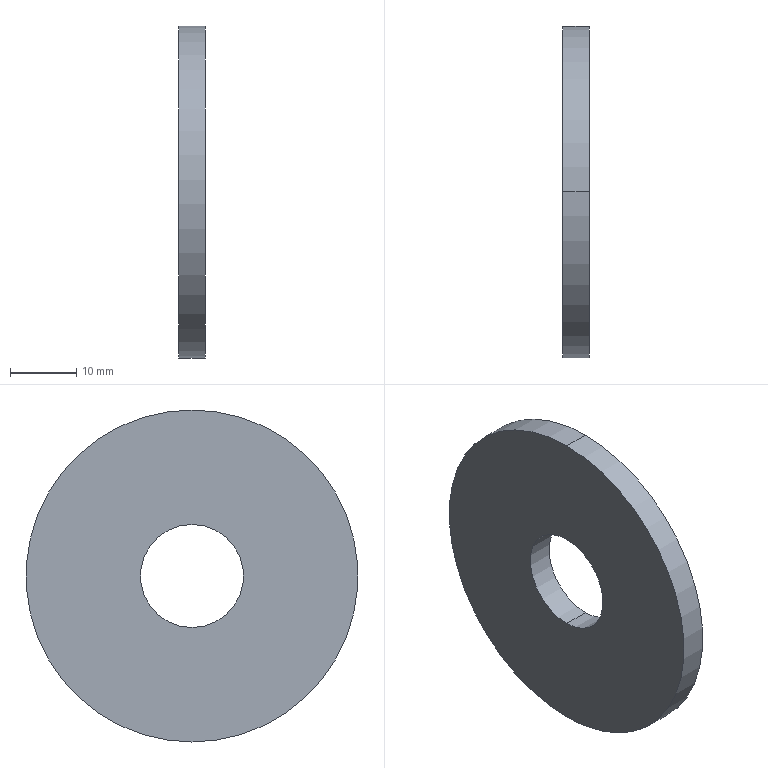Part | STEP file | flat washer wide_am_B18.22M - Plain washer, 14 mm, wide | 1 solid | 6 faces | box 4 x 50 x 50 mm | volume 7097 mm3 | cylinder 4 | plane 2 | commonest cylinder face diameters 15.52 x2 50 x2
STEP:
#1=CARTESIAN_POINT('',(0.,0.,0.));
#2=DIRECTION('',(0.,0.,1.));
#3=DIRECTION('',(1.,0.,0.));
#4=AXIS2_PLACEMENT_3D('',#1,#2,#3);
#5=CARTESIAN_POINT('',(0.,0.,25.));
#6=VERTEX_POINT('',#5);
#7=CARTESIAN_POINT('',(0.,0.,-25.));
#8=VERTEX_POINT('',#7);
#9=CARTESIAN_POINT('',(0.,0.,0.));
#10=DIRECTION('',(-1.,0.,0.));
#11=DIRECTION('',(0.,0.,1.));
#12=AXIS2_PLACEMENT_3D('',#9,#10,#11);
#13=CIRCLE('',#12,25.);
#14=CARTESIAN_POINT('',(-34.925,0.,0.));
#15=DIRECTION('',(-1.,0.,0.));
#16=DIRECTION('',(0.,0.,1.));
#17=AXIS2_PLACEMENT_3D('',#14,#15,#16);
#18=CYLINDRICAL_SURFACE('',#17,25.);
#19=CARTESIAN_POINT('',(0.,-34.925));
#20=DIRECTION('',(1.,0.));
#21=VECTOR('',#20,1.);
#22=LINE('',#19,#21);
#23=(GEOMETRIC_REPRESENTATION_CONTEXT(2)PARAMETRIC_REPRESENTATION_CONTEXT()REPRESENTATION_CONTEXT('',''));
#24=DEFINITIONAL_REPRESENTATION('',(#22),#23);
#25=PCURVE('',#18,#24);
#26=CARTESIAN_POINT('',(0.,7.76,0.));
#27=DIRECTION('',(-1.,0.,0.));
#28=DIRECTION('',(0.,0.,1.));
#29=AXIS2_PLACEMENT_3D('',#26,#27,#28);
#30=PLANE('',#29);
#31=CARTESIAN_POINT('',(0.,-7.76));
#32=DIRECTION('',(1.,0.));
#33=AXIS2_PLACEMENT_2D('',#31,#32);
#34=CIRCLE('',#33,25.);
#35=(GEOMETRIC_REPRESENTATION_CONTEXT(2)PARAMETRIC_REPRESENTATION_CONTEXT()REPRESENTATION_CONTEXT('',''));
#36=DEFINITIONAL_REPRESENTATION('',(#34),#35);
#37=PCURVE('',#30,#36);
#38=SURFACE_CURVE('',#13,(#25,#37),.PCURVE_S1.);
#39=EDGE_CURVE('',#6,#8,#38,.T.);
#40=ORIENTED_EDGE('',*,*,#39,.T.);
#41=CARTESIAN_POINT('',(-4.,0.,-25.));
#42=VERTEX_POINT('',#41);
#43=CARTESIAN_POINT('',(-34.925,0.,-25.));
#44=DIRECTION('',(-1.,0.,0.));
#45=VECTOR('',#44,1.);
#46=LINE('',#43,#45);
#47=CARTESIAN_POINT('',(3.142,0.));
#48=DIRECTION('',(0.,1.));
#49=VECTOR('',#48,1.);
#50=LINE('',#47,#49);
#51=(GEOMETRIC_REPRESENTATION_CONTEXT(2)PARAMETRIC_REPRESENTATION_CONTEXT()REPRESENTATION_CONTEXT('',''));
#52=DEFINITIONAL_REPRESENTATION('',(#50),#51);
#53=PCURVE('',#18,#52);
#54=CARTESIAN_POINT('',(-34.925,0.,0.));
#55=DIRECTION('',(-1.,0.,0.));
#56=DIRECTION('',(0.,0.,1.));
#57=AXIS2_PLACEMENT_3D('',#54,#55,#56);
#58=CYLINDRICAL_SURFACE('',#57,25.);
#59=CARTESIAN_POINT('',(3.142,0.));
#60=DIRECTION('',(0.,1.));
#61=VECTOR('',#60,1.);
#62=LINE('',#59,#61);
#63=(GEOMETRIC_REPRESENTATION_CONTEXT(2)PARAMETRIC_REPRESENTATION_CONTEXT()REPRESENTATION_CONTEXT('',''));
#64=DEFINITIONAL_REPRESENTATION('',(#62),#63);
#65=PCURVE('',#58,#64);
#66=SURFACE_CURVE('',#46,(#53,#65),.PCURVE_S1.);
#67=EDGE_CURVE('',#8,#42,#66,.T.);
#68=ORIENTED_EDGE('',*,*,#67,.T.);
#69=CARTESIAN_POINT('',(-4.,0.,25.));
#70=VERTEX_POINT('',#69);
#71=CARTESIAN_POINT('',(-4.,0.,0.));
#72=DIRECTION('',(-1.,0.,0.));
#73=DIRECTION('',(0.,0.,1.));
#74=AXIS2_PLACEMENT_3D('',#71,#72,#73);
#75=CIRCLE('',#74,25.);
#76=CARTESIAN_POINT('',(0.,-30.925));
#77=DIRECTION('',(1.,0.));
#78=VECTOR('',#77,1.);
#79=LINE('',#76,#78);
#80=(GEOMETRIC_REPRESENTATION_CONTEXT(2)PARAMETRIC_REPRESENTATION_CONTEXT()REPRESENTATION_CONTEXT('',''));
#81=DEFINITIONAL_REPRESENTATION('',(#79),#80);
#82=PCURVE('',#18,#81);
#83=CARTESIAN_POINT('',(-4.,25.,0.));
#84=DIRECTION('',(1.,0.,0.));
#85=DIRECTION('',(0.,0.,-1.));
#86=AXIS2_PLACEMENT_3D('',#83,#84,#85);
#87=PLANE('',#86);
#88=CARTESIAN_POINT('',(-25.,-25.));
#89=CARTESIAN_POINT('',(-25.,18.301));
#90=CARTESIAN_POINT('',(12.5,-3.349));
#91=CARTESIAN_POINT('',(50.,-25.));
#92=CARTESIAN_POINT('',(12.5,-46.651));
#93=CARTESIAN_POINT('',(-25.,-68.301));
#94=CARTESIAN_POINT('',(-25.,-25.));
#95=(BOUNDED_CURVE()B_SPLINE_CURVE(2,(#88,#89,#90,#91,#92,#93,#94),.UNSPECIFIED.,.T.,.F.)B_SPLINE_CURVE_WITH_KNOTS((1,2,2,2,2,1),(-2.094,0.,2.094,4.189,6.283,8.378),.UNSPECIFIED.)CURVE()GEOMETRIC_REPRESENTATION_ITEM()RATIONAL_B_SPLINE_CURVE((1.,0.5,1.,0.5,1.,0.5,1.))REPRESENTATION_ITEM(''));
#96=(GEOMETRIC_REPRESENTATION_CONTEXT(2)PARAMETRIC_REPRESENTATION_CONTEXT()REPRESENTATION_CONTEXT('',''));
#97=DEFINITIONAL_REPRESENTATION('',(#95),#96);
#98=PCURVE('',#87,#97);
#99=SURFACE_CURVE('',#75,(#82,#98),.PCURVE_S1.);
#100=EDGE_CURVE('',#70,#42,#99,.T.);
#101=ORIENTED_EDGE('',*,*,#100,.F.);
#102=CARTESIAN_POINT('',(-34.925,0.,25.));
#103=DIRECTION('',(-1.,0.,0.));
#104=VECTOR('',#103,1.);
#105=LINE('',#102,#104);
#106=CARTESIAN_POINT('',(0.,0.));
#107=DIRECTION('',(0.,1.));
#108=VECTOR('',#107,1.);
#109=LINE('',#106,#108);
#110=(GEOMETRIC_REPRESENTATION_CONTEXT(2)PARAMETRIC_REPRESENTATION_CONTEXT()REPRESENTATION_CONTEXT('',''));
#111=DEFINITIONAL_REPRESENTATION('',(#109),#110);
#112=PCURVE('',#18,#111);
#113=CARTESIAN_POINT('',(6.283,0.));
#114=DIRECTION('',(0.,1.));
#115=VECTOR('',#114,1.);
#116=LINE('',#113,#115);
#117=(GEOMETRIC_REPRESENTATION_CONTEXT(2)PARAMETRIC_REPRESENTATION_CONTEXT()REPRESENTATION_CONTEXT('',''));
#118=DEFINITIONAL_REPRESENTATION('',(#116),#117);
#119=PCURVE('',#58,#118);
#120=SURFACE_CURVE('',#105,(#112,#119),.PCURVE_S1.);
#121=EDGE_CURVE('',#6,#70,#120,.T.);
#122=ORIENTED_EDGE('',*,*,#121,.F.);
#123=EDGE_LOOP('',(#40,#68,#101,#122));
#124=FACE_BOUND('',#123,.T.);
#125=ADVANCED_FACE('',(#124),#18,.T.);
#126=CARTESIAN_POINT('',(0.,0.,7.76));
#127=VERTEX_POINT('',#126);
#128=CARTESIAN_POINT('',(-4.,0.,7.76));
#129=VERTEX_POINT('',#128);
#130=CARTESIAN_POINT('',(-34.925,0.,7.76));
#131=DIRECTION('',(-1.,0.,0.));
#132=VECTOR('',#131,1.);
#133=LINE('',#130,#132);
#134=CARTESIAN_POINT('',(-34.925,0.,0.));
#135=DIRECTION('',(-1.,0.,0.));
#136=DIRECTION('',(0.,0.,1.));
#137=AXIS2_PLACEMENT_3D('',#134,#135,#136);
#138=CYLINDRICAL_SURFACE('',#137,7.76);
#139=CARTESIAN_POINT('',(6.283,0.));
#140=DIRECTION('',(0.,1.));
#141=VECTOR('',#140,1.);
#142=LINE('',#139,#141);
#143=(GEOMETRIC_REPRESENTATION_CONTEXT(2)PARAMETRIC_REPRESENTATION_CONTEXT()REPRESENTATION_CONTEXT('',''));
#144=DEFINITIONAL_REPRESENTATION('',(#142),#143);
#145=PCURVE('',#138,#144);
#146=CARTESIAN_POINT('',(-34.925,0.,0.));
#147=DIRECTION('',(-1.,0.,0.));
#148=DIRECTION('',(0.,0.,1.));
#149=AXIS2_PLACEMENT_3D('',#146,#147,#148);
#150=CYLINDRICAL_SURFACE('',#149,7.76);
#151=CARTESIAN_POINT('',(0.,0.));
#152=DIRECTION('',(0.,1.));
#153=VECTOR('',#152,1.);
#154=LINE('',#151,#153);
#155=(GEOMETRIC_REPRESENTATION_CONTEXT(2)PARAMETRIC_REPRESENTATION_CONTEXT()REPRESENTATION_CONTEXT('',''));
#156=DEFINITIONAL_REPRESENTATION('',(#154),#155);
#157=PCURVE('',#150,#156);
#158=SURFACE_CURVE('',#133,(#145,#157),.PCURVE_S1.);
#159=EDGE_CURVE('',#127,#129,#158,.T.);
#160=ORIENTED_EDGE('',*,*,#159,.T.);
#161=CARTESIAN_POINT('',(-4.,0.,-7.76));
#162=VERTEX_POINT('',#161);
#163=CARTESIAN_POINT('',(-4.,0.,0.));
#164=DIRECTION('',(-1.,0.,0.));
#165=DIRECTION('',(0.,0.,1.));
#166=AXIS2_PLACEMENT_3D('',#163,#164,#165);
#167=CIRCLE('',#166,7.76);
#168=CARTESIAN_POINT('',(0.,-30.925));
#169=DIRECTION('',(1.,0.));
#170=VECTOR('',#169,1.);
#171=LINE('',#168,#170);
#172=(GEOMETRIC_REPRESENTATION_CONTEXT(2)PARAMETRIC_REPRESENTATION_CONTEXT()REPRESENTATION_CONTEXT('',''));
#173=DEFINITIONAL_REPRESENTATION('',(#171),#172);
#174=PCURVE('',#138,#173);
#175=CARTESIAN_POINT('',(-7.76,-25.));
#176=CARTESIAN_POINT('',(-7.76,-11.559));
#177=CARTESIAN_POINT('',(3.88,-18.28));
#178=CARTESIAN_POINT('',(15.52,-25.));
#179=CARTESIAN_POINT('',(3.88,-31.72));
#180=CARTESIAN_POINT('',(-7.76,-38.441));
#181=CARTESIAN_POINT('',(-7.76,-25.));
#182=(BOUNDED_CURVE()B_SPLINE_CURVE(2,(#175,#176,#177,#178,#179,#180,#181),.UNSPECIFIED.,.T.,.F.)B_SPLINE_CURVE_WITH_KNOTS((1,2,2,2,2,1),(-2.094,0.,2.094,4.189,6.283,8.378),.UNSPECIFIED.)CURVE()GEOMETRIC_REPRESENTATION_ITEM()RATIONAL_B_SPLINE_CURVE((1.,0.5,1.,0.5,1.,0.5,1.))REPRESENTATION_ITEM(''));
#183=(GEOMETRIC_REPRESENTATION_CONTEXT(2)PARAMETRIC_REPRESENTATION_CONTEXT()REPRESENTATION_CONTEXT('',''));
#184=DEFINITIONAL_REPRESENTATION('',(#182),#183);
#185=PCURVE('',#87,#184);
#186=SURFACE_CURVE('',#167,(#174,#185),.PCURVE_S1.);
#187=EDGE_CURVE('',#162,#129,#186,.T.);
#188=ORIENTED_EDGE('',*,*,#187,.F.);
#189=CARTESIAN_POINT('',(0.,0.,-7.76));
#190=VERTEX_POINT('',#189);
#191=CARTESIAN_POINT('',(-34.925,0.,-7.76));
#192=DIRECTION('',(-1.,0.,0.));
#193=VECTOR('',#192,1.);
#194=LINE('',#191,#193);
#195=CARTESIAN_POINT('',(3.142,0.));
#196=DIRECTION('',(0.,1.));
#197=VECTOR('',#196,1.);
#198=LINE('',#195,#197);
#199=(GEOMETRIC_REPRESENTATION_CONTEXT(2)PARAMETRIC_REPRESENTATION_CONTEXT()REPRESENTATION_CONTEXT('',''));
#200=DEFINITIONAL_REPRESENTATION('',(#198),#199);
#201=PCURVE('',#138,#200);
#202=CARTESIAN_POINT('',(3.142,0.));
#203=DIRECTION('',(0.,1.));
#204=VECTOR('',#203,1.);
#205=LINE('',#202,#204);
#206=(GEOMETRIC_REPRESENTATION_CONTEXT(2)PARAMETRIC_REPRESENTATION_CONTEXT()REPRESENTATION_CONTEXT('',''));
#207=DEFINITIONAL_REPRESENTATION('',(#205),#206);
#208=PCURVE('',#150,#207);
#209=SURFACE_CURVE('',#194,(#201,#208),.PCURVE_S1.);
#210=EDGE_CURVE('',#190,#162,#209,.T.);
#211=ORIENTED_EDGE('',*,*,#210,.F.);
#212=CARTESIAN_POINT('',(0.,0.,0.));
#213=DIRECTION('',(-1.,0.,0.));
#214=DIRECTION('',(0.,0.,1.));
#215=AXIS2_PLACEMENT_3D('',#212,#213,#214);
#216=CIRCLE('',#215,7.76);
#217=CARTESIAN_POINT('',(0.,-34.925));
#218=DIRECTION('',(1.,0.));
#219=VECTOR('',#218,1.);
#220=LINE('',#217,#219);
#221=(GEOMETRIC_REPRESENTATION_CONTEXT(2)PARAMETRIC_REPRESENTATION_CONTEXT()REPRESENTATION_CONTEXT('',''));
#222=DEFINITIONAL_REPRESENTATION('',(#220),#221);
#223=PCURVE('',#138,#222);
#224=CARTESIAN_POINT('',(0.,-7.76));
#225=DIRECTION('',(1.,0.));
#226=AXIS2_PLACEMENT_2D('',#224,#225);
#227=CIRCLE('',#226,7.76);
#228=(GEOMETRIC_REPRESENTATION_CONTEXT(2)PARAMETRIC_REPRESENTATION_CONTEXT()REPRESENTATION_CONTEXT('',''));
#229=DEFINITIONAL_REPRESENTATION('',(#227),#228);
#230=PCURVE('',#30,#229);
#231=SURFACE_CURVE('',#216,(#223,#230),.PCURVE_S1.);
#232=EDGE_CURVE('',#190,#127,#231,.T.);
#233=ORIENTED_EDGE('',*,*,#232,.T.);
#234=EDGE_LOOP('',(#160,#188,#211,#233));
#235=FACE_BOUND('',#234,.F.);
#236=ADVANCED_FACE('',(#235),#138,.F.);
#237=CARTESIAN_POINT('',(-4.,0.,0.));
#238=DIRECTION('',(-1.,0.,0.));
#239=DIRECTION('',(0.,0.,1.));
#240=AXIS2_PLACEMENT_3D('',#237,#238,#239);
#241=CIRCLE('',#240,7.76);
#242=CARTESIAN_POINT('',(0.,-30.925));
#243=DIRECTION('',(1.,0.));
#244=VECTOR('',#243,1.);
#245=LINE('',#242,#244);
#246=(GEOMETRIC_REPRESENTATION_CONTEXT(2)PARAMETRIC_REPRESENTATION_CONTEXT()REPRESENTATION_CONTEXT('',''));
#247=DEFINITIONAL_REPRESENTATION('',(#245),#246);
#248=PCURVE('',#150,#247);
#249=CARTESIAN_POINT('',(-7.76,-25.));
#250=CARTESIAN_POINT('',(-7.76,-11.559));
#251=CARTESIAN_POINT('',(3.88,-18.28));
#252=CARTESIAN_POINT('',(15.52,-25.));
#253=CARTESIAN_POINT('',(3.88,-31.72));
#254=CARTESIAN_POINT('',(-7.76,-38.441));
#255=CARTESIAN_POINT('',(-7.76,-25.));
#256=(BOUNDED_CURVE()B_SPLINE_CURVE(2,(#249,#250,#251,#252,#253,#254,#255),.UNSPECIFIED.,.T.,.F.)B_SPLINE_CURVE_WITH_KNOTS((1,2,2,2,2,1),(-2.094,0.,2.094,4.189,6.283,8.378),.UNSPECIFIED.)CURVE()GEOMETRIC_REPRESENTATION_ITEM()RATIONAL_B_SPLINE_CURVE((1.,0.5,1.,0.5,1.,0.5,1.))REPRESENTATION_ITEM(''));
#257=(GEOMETRIC_REPRESENTATION_CONTEXT(2)PARAMETRIC_REPRESENTATION_CONTEXT()REPRESENTATION_CONTEXT('',''));
#258=DEFINITIONAL_REPRESENTATION('',(#256),#257);
#259=PCURVE('',#87,#258);
#260=SURFACE_CURVE('',#241,(#248,#259),.PCURVE_S1.);
#261=EDGE_CURVE('',#129,#162,#260,.T.);
#262=ORIENTED_EDGE('',*,*,#261,.F.);
#263=ORIENTED_EDGE('',*,*,#159,.F.);
#264=CARTESIAN_POINT('',(0.,0.,0.));
#265=DIRECTION('',(-1.,0.,0.));
#266=DIRECTION('',(0.,0.,1.));
#267=AXIS2_PLACEMENT_3D('',#264,#265,#266);
#268=CIRCLE('',#267,7.76);
#269=CARTESIAN_POINT('',(0.,-34.925));
#270=DIRECTION('',(1.,0.));
#271=VECTOR('',#270,1.);
#272=LINE('',#269,#271);
#273=(GEOMETRIC_REPRESENTATION_CONTEXT(2)PARAMETRIC_REPRESENTATION_CONTEXT()REPRESENTATION_CONTEXT('',''));
#274=DEFINITIONAL_REPRESENTATION('',(#272),#273);
#275=PCURVE('',#150,#274);
#276=CARTESIAN_POINT('',(0.,-7.76));
#277=DIRECTION('',(1.,0.));
#278=AXIS2_PLACEMENT_2D('',#276,#277);
#279=CIRCLE('',#278,7.76);
#280=(GEOMETRIC_REPRESENTATION_CONTEXT(2)PARAMETRIC_REPRESENTATION_CONTEXT()REPRESENTATION_CONTEXT('',''));
#281=DEFINITIONAL_REPRESENTATION('',(#279),#280);
#282=PCURVE('',#30,#281);
#283=SURFACE_CURVE('',#268,(#275,#282),.PCURVE_S1.);
#284=EDGE_CURVE('',#127,#190,#283,.T.);
#285=ORIENTED_EDGE('',*,*,#284,.T.);
#286=ORIENTED_EDGE('',*,*,#210,.T.);
#287=EDGE_LOOP('',(#262,#263,#285,#286));
#288=FACE_BOUND('',#287,.F.);
#289=ADVANCED_FACE('',(#288),#150,.F.);
#290=ORIENTED_EDGE('',*,*,#39,.F.);
#291=CARTESIAN_POINT('',(0.,0.,0.));
#292=DIRECTION('',(-1.,0.,0.));
#293=DIRECTION('',(0.,0.,1.));
#294=AXIS2_PLACEMENT_3D('',#291,#292,#293);
#295=CIRCLE('',#294,25.);
#296=CARTESIAN_POINT('',(0.,-7.76));
#297=DIRECTION('',(1.,0.));
#298=AXIS2_PLACEMENT_2D('',#296,#297);
#299=CIRCLE('',#298,25.);
#300=(GEOMETRIC_REPRESENTATION_CONTEXT(2)PARAMETRIC_REPRESENTATION_CONTEXT()REPRESENTATION_CONTEXT('',''));
#301=DEFINITIONAL_REPRESENTATION('',(#299),#300);
#302=PCURVE('',#30,#301);
#303=CARTESIAN_POINT('',(0.,-34.925));
#304=DIRECTION('',(1.,0.));
#305=VECTOR('',#304,1.);
#306=LINE('',#303,#305);
#307=(GEOMETRIC_REPRESENTATION_CONTEXT(2)PARAMETRIC_REPRESENTATION_CONTEXT()REPRESENTATION_CONTEXT('',''));
#308=DEFINITIONAL_REPRESENTATION('',(#306),#307);
#309=PCURVE('',#58,#308);
#310=SURFACE_CURVE('',#295,(#302,#309),.PCURVE_S1.);
#311=EDGE_CURVE('',#8,#6,#310,.T.);
#312=ORIENTED_EDGE('',*,*,#311,.F.);
#313=EDGE_LOOP('',(#290,#312));
#314=FACE_BOUND('',#313,.T.);
#315=ORIENTED_EDGE('',*,*,#284,.T.);
#316=ORIENTED_EDGE('',*,*,#232,.T.);
#317=EDGE_LOOP('',(#315,#316));
#318=FACE_BOUND('',#317,.T.);
#319=ADVANCED_FACE('',(#314,#318),#30,.F.);
#320=ORIENTED_EDGE('',*,*,#67,.F.);
#321=ORIENTED_EDGE('',*,*,#311,.T.);
#322=ORIENTED_EDGE('',*,*,#121,.T.);
#323=CARTESIAN_POINT('',(-4.,0.,0.));
#324=DIRECTION('',(-1.,0.,0.));
#325=DIRECTION('',(0.,0.,1.));
#326=AXIS2_PLACEMENT_3D('',#323,#324,#325);
#327=CIRCLE('',#326,25.);
#328=CARTESIAN_POINT('',(0.,-30.925));
#329=DIRECTION('',(1.,0.));
#330=VECTOR('',#329,1.);
#331=LINE('',#328,#330);
#332=(GEOMETRIC_REPRESENTATION_CONTEXT(2)PARAMETRIC_REPRESENTATION_CONTEXT()REPRESENTATION_CONTEXT('',''));
#333=DEFINITIONAL_REPRESENTATION('',(#331),#332);
#334=PCURVE('',#58,#333);
#335=CARTESIAN_POINT('',(-25.,-25.));
#336=CARTESIAN_POINT('',(-25.,18.301));
#337=CARTESIAN_POINT('',(12.5,-3.349));
#338=CARTESIAN_POINT('',(50.,-25.));
#339=CARTESIAN_POINT('',(12.5,-46.651));
#340=CARTESIAN_POINT('',(-25.,-68.301));
#341=CARTESIAN_POINT('',(-25.,-25.));
#342=(BOUNDED_CURVE()B_SPLINE_CURVE(2,(#335,#336,#337,#338,#339,#340,#341),.UNSPECIFIED.,.T.,.F.)B_SPLINE_CURVE_WITH_KNOTS((1,2,2,2,2,1),(-2.094,0.,2.094,4.189,6.283,8.378),.UNSPECIFIED.)CURVE()GEOMETRIC_REPRESENTATION_ITEM()RATIONAL_B_SPLINE_CURVE((1.,0.5,1.,0.5,1.,0.5,1.))REPRESENTATION_ITEM(''));
#343=(GEOMETRIC_REPRESENTATION_CONTEXT(2)PARAMETRIC_REPRESENTATION_CONTEXT()REPRESENTATION_CONTEXT('',''));
#344=DEFINITIONAL_REPRESENTATION('',(#342),#343);
#345=PCURVE('',#87,#344);
#346=SURFACE_CURVE('',#327,(#334,#345),.PCURVE_S1.);
#347=EDGE_CURVE('',#42,#70,#346,.T.);
#348=ORIENTED_EDGE('',*,*,#347,.F.);
#349=EDGE_LOOP('',(#320,#321,#322,#348));
#350=FACE_BOUND('',#349,.T.);
#351=ADVANCED_FACE('',(#350),#58,.T.);
#352=ORIENTED_EDGE('',*,*,#261,.F.);
#353=ORIENTED_EDGE('',*,*,#187,.F.);
#354=EDGE_LOOP('',(#352,#353));
#355=FACE_BOUND('',#354,.T.);
#356=ORIENTED_EDGE('',*,*,#100,.T.);
#357=ORIENTED_EDGE('',*,*,#347,.T.);
#358=EDGE_LOOP('',(#356,#357));
#359=FACE_BOUND('',#358,.T.);
#360=ADVANCED_FACE('',(#355,#359),#87,.F.);
#361=CLOSED_SHELL('',(#125,#236,#289,#319,#351,#360));
#362=MANIFOLD_SOLID_BREP('',#361);
#363=(LENGTH_UNIT()NAMED_UNIT(*)SI_UNIT(.MILLI.,.METRE.));
#364=UNCERTAINTY_MEASURE_WITH_UNIT(LENGTH_MEASURE(0.0000001),#363,'','');
#365=(NAMED_UNIT(*)PLANE_ANGLE_UNIT()SI_UNIT($,.RADIAN.));
#366=(NAMED_UNIT(*)SI_UNIT($,.STERADIAN.)SOLID_ANGLE_UNIT());
#367=(GEOMETRIC_REPRESENTATION_CONTEXT(3)GLOBAL_UNCERTAINTY_ASSIGNED_CONTEXT((#364))GLOBAL_UNIT_ASSIGNED_CONTEXT((#363,#365,#366))REPRESENTATION_CONTEXT('',''));
#368=ADVANCED_BREP_SHAPE_REPRESENTATION('',(#4,#362),#367);